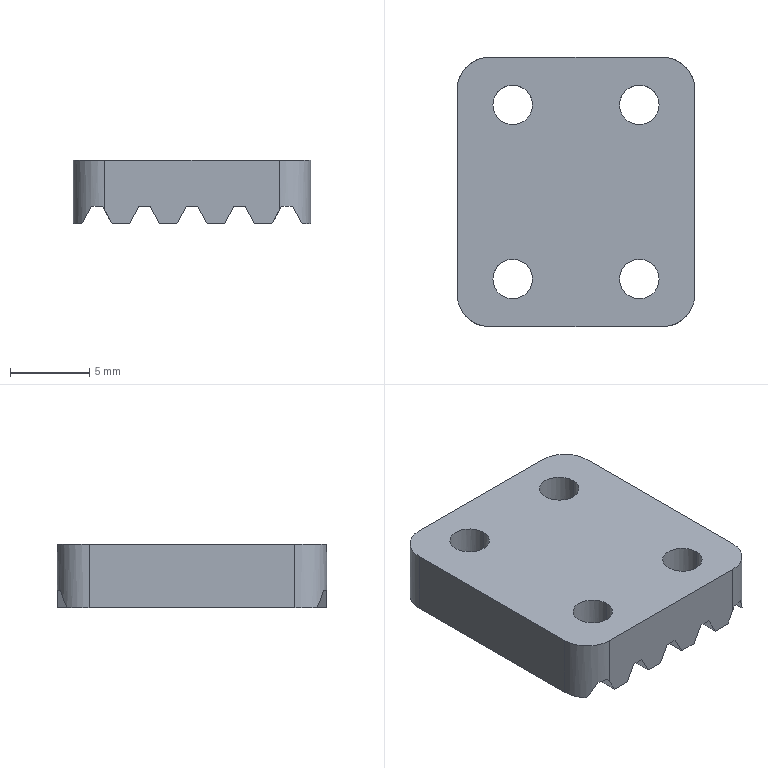Part | NX | features BREP 1 | 1 solid | 46 faces | box 15 x 17 x 4 mm | volume 813.959 mm3 | plane 34 | cylinder 12 | commonest cylinder face diameters 2.5 x8 4 x4